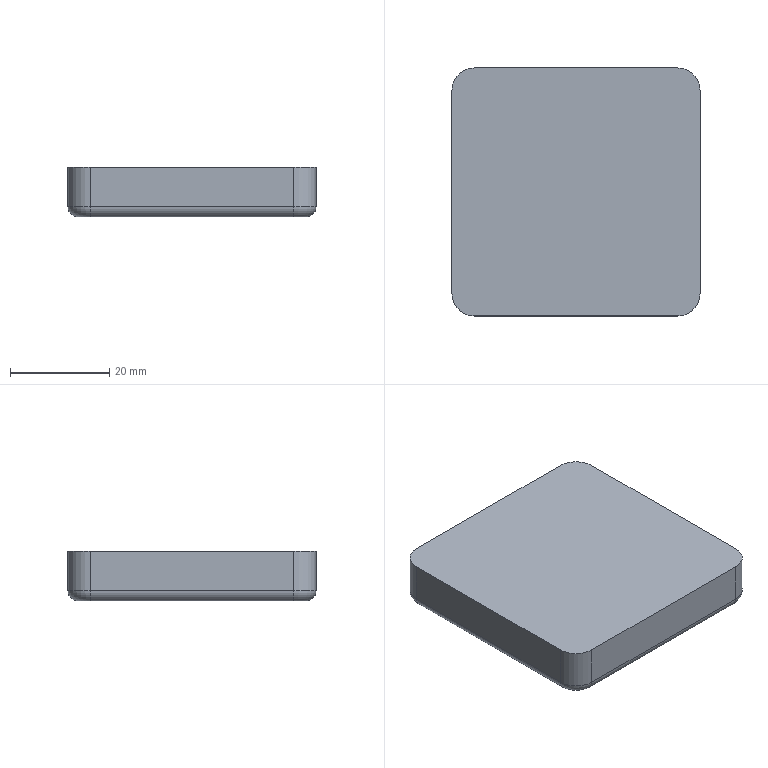Part | STEP file | 14831_CPY | 1 solid | 18 faces | box 50 x 50 x 10 mm | volume 24664 mm3 | cylinder 8 | plane 6 | torus 4 | commonest cylinder face diameters 4 x4 9 x4
STEP:
#1=CARTESIAN_POINT('',(0.,0.,0.));
#2=DIRECTION('',(0.,0.,1.));
#3=DIRECTION('',(1.,0.,0.));
#4=AXIS2_PLACEMENT_3D('',#1,#2,#3);
#5=CARTESIAN_POINT('',(-133.276,-146.636,0.));
#6=VERTEX_POINT('',#5);
#7=CARTESIAN_POINT('',(-133.276,-148.636,2.));
#8=VERTEX_POINT('',#7);
#9=CARTESIAN_POINT('',(-133.276,-146.636,2.));
#10=DIRECTION('',(-1.,0.,0.));
#11=DIRECTION('',(0.,0.,-1.));
#12=AXIS2_PLACEMENT_3D('',#9,#10,#11);
#13=CIRCLE('',#12,2.);
#14=CARTESIAN_POINT('',(-143.526,-146.636,2.));
#15=DIRECTION('',(-1.,0.,0.));
#16=DIRECTION('',(0.,-0.7071,-0.7071));
#17=AXIS2_PLACEMENT_3D('',#14,#15,#16);
#18=CYLINDRICAL_SURFACE('',#17,2.);
#19=CARTESIAN_POINT('',(5.498,-10.25));
#20=DIRECTION('',(1.,0.));
#21=VECTOR('',#20,1.);
#22=LINE('',#19,#21);
#23=(GEOMETRIC_REPRESENTATION_CONTEXT(2)PARAMETRIC_REPRESENTATION_CONTEXT()REPRESENTATION_CONTEXT('',''));
#24=DEFINITIONAL_REPRESENTATION('',(#22),#23);
#25=PCURVE('',#18,#24);
#26=CARTESIAN_POINT('',(-133.276,-144.136,2.));
#27=DIRECTION('',(0.,0.,-1.));
#28=DIRECTION('',(-1.,0.,0.));
#29=AXIS2_PLACEMENT_3D('',#26,#27,#28);
#30=TOROIDAL_SURFACE('',#29,2.5,2.);
#31=CARTESIAN_POINT('',(4.712,1.571));
#32=DIRECTION('',(0.,-1.));
#33=VECTOR('',#32,1.);
#34=LINE('',#31,#33);
#35=(GEOMETRIC_REPRESENTATION_CONTEXT(2)PARAMETRIC_REPRESENTATION_CONTEXT()REPRESENTATION_CONTEXT('',''));
#36=DEFINITIONAL_REPRESENTATION('',(#34),#35);
#37=PCURVE('',#30,#36);
#38=SURFACE_CURVE('',#13,(#25,#37),.PCURVE_S1.);
#39=EDGE_CURVE('',#6,#8,#38,.T.);
#40=ORIENTED_EDGE('',*,*,#39,.T.);
#41=CARTESIAN_POINT('',(-174.276,-148.636,2.));
#42=VERTEX_POINT('',#41);
#43=CARTESIAN_POINT('',(-133.276,-148.636,2.));
#44=DIRECTION('',(-1.,0.,0.));
#45=VECTOR('',#44,1.);
#46=LINE('',#43,#45);
#47=CARTESIAN_POINT('',(7.069,-10.25));
#48=DIRECTION('',(0.,1.));
#49=VECTOR('',#48,1.);
#50=LINE('',#47,#49);
#51=(GEOMETRIC_REPRESENTATION_CONTEXT(2)PARAMETRIC_REPRESENTATION_CONTEXT()REPRESENTATION_CONTEXT('',''));
#52=DEFINITIONAL_REPRESENTATION('',(#50),#51);
#53=PCURVE('',#18,#52);
#54=CARTESIAN_POINT('',(-133.276,-148.636,0.));
#55=DIRECTION('',(0.,-1.,0.));
#56=DIRECTION('',(0.,0.,-1.));
#57=AXIS2_PLACEMENT_3D('',#54,#55,#56);
#58=PLANE('',#57);
#59=CARTESIAN_POINT('',(-2.,0.));
#60=DIRECTION('',(0.,-1.));
#61=VECTOR('',#60,1.);
#62=LINE('',#59,#61);
#63=(GEOMETRIC_REPRESENTATION_CONTEXT(2)PARAMETRIC_REPRESENTATION_CONTEXT()REPRESENTATION_CONTEXT('',''));
#64=DEFINITIONAL_REPRESENTATION('',(#62),#63);
#65=PCURVE('',#58,#64);
#66=SURFACE_CURVE('',#46,(#53,#65),.PCURVE_S1.);
#67=EDGE_CURVE('',#8,#42,#66,.T.);
#68=ORIENTED_EDGE('',*,*,#67,.T.);
#69=CARTESIAN_POINT('',(-174.276,-146.636,0.));
#70=VERTEX_POINT('',#69);
#71=CARTESIAN_POINT('',(-174.276,-146.636,2.));
#72=DIRECTION('',(1.,0.,0.));
#73=DIRECTION('',(0.,-1.,0.));
#74=AXIS2_PLACEMENT_3D('',#71,#72,#73);
#75=CIRCLE('',#74,2.);
#76=CARTESIAN_POINT('',(7.069,30.75));
#77=DIRECTION('',(-1.,0.));
#78=VECTOR('',#77,1.);
#79=LINE('',#76,#78);
#80=(GEOMETRIC_REPRESENTATION_CONTEXT(2)PARAMETRIC_REPRESENTATION_CONTEXT()REPRESENTATION_CONTEXT('',''));
#81=DEFINITIONAL_REPRESENTATION('',(#79),#80);
#82=PCURVE('',#18,#81);
#83=CARTESIAN_POINT('',(-174.276,-144.136,2.));
#84=DIRECTION('',(0.,0.,-1.));
#85=DIRECTION('',(-1.,0.,0.));
#86=AXIS2_PLACEMENT_3D('',#83,#84,#85);
#87=TOROIDAL_SURFACE('',#86,2.5,2.);
#88=CARTESIAN_POINT('',(4.712,0.));
#89=DIRECTION('',(0.,1.));
#90=VECTOR('',#89,1.);
#91=LINE('',#88,#90);
#92=(GEOMETRIC_REPRESENTATION_CONTEXT(2)PARAMETRIC_REPRESENTATION_CONTEXT()REPRESENTATION_CONTEXT('',''));
#93=DEFINITIONAL_REPRESENTATION('',(#91),#92);
#94=PCURVE('',#87,#93);
#95=SURFACE_CURVE('',#75,(#82,#94),.PCURVE_S1.);
#96=EDGE_CURVE('',#42,#70,#95,.T.);
#97=ORIENTED_EDGE('',*,*,#96,.T.);
#98=CARTESIAN_POINT('',(-174.276,-146.636,0.));
#99=DIRECTION('',(1.,0.,0.));
#100=VECTOR('',#99,1.);
#101=LINE('',#98,#100);
#102=CARTESIAN_POINT('',(5.498,30.75));
#103=DIRECTION('',(0.,-1.));
#104=VECTOR('',#103,1.);
#105=LINE('',#102,#104);
#106=(GEOMETRIC_REPRESENTATION_CONTEXT(2)PARAMETRIC_REPRESENTATION_CONTEXT()REPRESENTATION_CONTEXT('',''));
#107=DEFINITIONAL_REPRESENTATION('',(#105),#106);
#108=PCURVE('',#18,#107);
#109=CARTESIAN_POINT('',(-153.776,-123.636,0.));
#110=DIRECTION('',(0.,0.,1.));
#111=DIRECTION('',(1.,0.,0.));
#112=AXIS2_PLACEMENT_3D('',#109,#110,#111);
#113=PLANE('',#112);
#114=CARTESIAN_POINT('',(-20.5,-23.));
#115=DIRECTION('',(1.,0.));
#116=VECTOR('',#115,1.);
#117=LINE('',#114,#116);
#118=(GEOMETRIC_REPRESENTATION_CONTEXT(2)PARAMETRIC_REPRESENTATION_CONTEXT()REPRESENTATION_CONTEXT('',''));
#119=DEFINITIONAL_REPRESENTATION('',(#117),#118);
#120=PCURVE('',#113,#119);
#121=SURFACE_CURVE('',#101,(#108,#120),.PCURVE_S1.);
#122=EDGE_CURVE('',#70,#6,#121,.T.);
#123=ORIENTED_EDGE('',*,*,#122,.T.);
#124=EDGE_LOOP('',(#40,#68,#97,#123));
#125=FACE_BOUND('',#124,.T.);
#126=ADVANCED_FACE('',(#125),#18,.T.);
#127=CARTESIAN_POINT('',(-130.776,-144.136,0.));
#128=VERTEX_POINT('',#127);
#129=CARTESIAN_POINT('',(-128.776,-144.136,2.));
#130=VERTEX_POINT('',#129);
#131=CARTESIAN_POINT('',(-130.776,-144.136,2.));
#132=DIRECTION('',(0.,-1.,0.));
#133=DIRECTION('',(0.,0.,-1.));
#134=AXIS2_PLACEMENT_3D('',#131,#132,#133);
#135=CIRCLE('',#134,2.);
#136=CARTESIAN_POINT('',(3.142,1.571));
#137=DIRECTION('',(0.,-1.));
#138=VECTOR('',#137,1.);
#139=LINE('',#136,#138);
#140=(GEOMETRIC_REPRESENTATION_CONTEXT(2)PARAMETRIC_REPRESENTATION_CONTEXT()REPRESENTATION_CONTEXT('',''));
#141=DEFINITIONAL_REPRESENTATION('',(#139),#140);
#142=PCURVE('',#30,#141);
#143=CARTESIAN_POINT('',(-130.776,-113.386,2.));
#144=DIRECTION('',(0.,-1.,0.));
#145=DIRECTION('',(0.7071,0.,-0.7071));
#146=AXIS2_PLACEMENT_3D('',#143,#144,#145);
#147=CYLINDRICAL_SURFACE('',#146,2.);
#148=CARTESIAN_POINT('',(5.498,30.75));
#149=DIRECTION('',(1.,0.));
#150=VECTOR('',#149,1.);
#151=LINE('',#148,#150);
#152=(GEOMETRIC_REPRESENTATION_CONTEXT(2)PARAMETRIC_REPRESENTATION_CONTEXT()REPRESENTATION_CONTEXT('',''));
#153=DEFINITIONAL_REPRESENTATION('',(#151),#152);
#154=PCURVE('',#147,#153);
#155=SURFACE_CURVE('',#135,(#142,#154),.PCURVE_S1.);
#156=EDGE_CURVE('',#128,#130,#155,.T.);
#157=ORIENTED_EDGE('',*,*,#156,.T.);
#158=CARTESIAN_POINT('',(-133.276,-144.136,2.));
#159=DIRECTION('',(0.,0.,-1.));
#160=DIRECTION('',(0.7071,-0.7071,0.));
#161=AXIS2_PLACEMENT_3D('',#158,#159,#160);
#162=CIRCLE('',#161,4.5);
#163=CARTESIAN_POINT('',(-2.356,0.));
#164=DIRECTION('',(1.,0.));
#165=VECTOR('',#164,1.);
#166=LINE('',#163,#165);
#167=(GEOMETRIC_REPRESENTATION_CONTEXT(2)PARAMETRIC_REPRESENTATION_CONTEXT()REPRESENTATION_CONTEXT('',''));
#168=DEFINITIONAL_REPRESENTATION('',(#166),#167);
#169=PCURVE('',#30,#168);
#170=CARTESIAN_POINT('',(-133.276,-144.136,0.));
#171=DIRECTION('',(0.,0.,1.));
#172=DIRECTION('',(0.,1.,0.));
#173=AXIS2_PLACEMENT_3D('',#170,#171,#172);
#174=CYLINDRICAL_SURFACE('',#173,4.5);
#175=CARTESIAN_POINT('',(10.21,2.));
#176=DIRECTION('',(-1.,0.));
#177=VECTOR('',#176,1.);
#178=LINE('',#175,#177);
#179=(GEOMETRIC_REPRESENTATION_CONTEXT(2)PARAMETRIC_REPRESENTATION_CONTEXT()REPRESENTATION_CONTEXT('',''));
#180=DEFINITIONAL_REPRESENTATION('',(#178),#179);
#181=PCURVE('',#174,#180);
#182=SURFACE_CURVE('',#162,(#169,#181),.PCURVE_S1.);
#183=EDGE_CURVE('',#130,#8,#182,.T.);
#184=ORIENTED_EDGE('',*,*,#183,.T.);
#185=ORIENTED_EDGE('',*,*,#39,.F.);
#186=CARTESIAN_POINT('',(-133.276,-144.136,0.));
#187=DIRECTION('',(0.,0.,1.));
#188=DIRECTION('',(0.7071,-0.7071,0.));
#189=AXIS2_PLACEMENT_3D('',#186,#187,#188);
#190=CIRCLE('',#189,2.5);
#191=CARTESIAN_POINT('',(10.21,1.571));
#192=DIRECTION('',(-1.,0.));
#193=VECTOR('',#192,1.);
#194=LINE('',#191,#193);
#195=(GEOMETRIC_REPRESENTATION_CONTEXT(2)PARAMETRIC_REPRESENTATION_CONTEXT()REPRESENTATION_CONTEXT('',''));
#196=DEFINITIONAL_REPRESENTATION('',(#194),#195);
#197=PCURVE('',#30,#196);
#198=CARTESIAN_POINT('',(20.5,-20.5));
#199=DIRECTION('',(0.7071,-0.7071));
#200=AXIS2_PLACEMENT_2D('',#198,#199);
#201=CIRCLE('',#200,2.5);
#202=(GEOMETRIC_REPRESENTATION_CONTEXT(2)PARAMETRIC_REPRESENTATION_CONTEXT()REPRESENTATION_CONTEXT('',''));
#203=DEFINITIONAL_REPRESENTATION('',(#201),#202);
#204=PCURVE('',#113,#203);
#205=SURFACE_CURVE('',#190,(#197,#204),.PCURVE_S1.);
#206=EDGE_CURVE('',#6,#128,#205,.T.);
#207=ORIENTED_EDGE('',*,*,#206,.T.);
#208=EDGE_LOOP('',(#157,#184,#185,#207));
#209=FACE_BOUND('',#208,.T.);
#210=ADVANCED_FACE('',(#209),#30,.T.);
#211=CARTESIAN_POINT('',(-178.776,-144.136,2.));
#212=VERTEX_POINT('',#211);
#213=CARTESIAN_POINT('',(-176.776,-144.136,0.));
#214=VERTEX_POINT('',#213);
#215=CARTESIAN_POINT('',(-176.776,-144.136,2.));
#216=DIRECTION('',(0.,-1.,0.));
#217=DIRECTION('',(-1.,0.,0.));
#218=AXIS2_PLACEMENT_3D('',#215,#216,#217);
#219=CIRCLE('',#218,2.);
#220=CARTESIAN_POINT('',(6.283,0.));
#221=DIRECTION('',(0.,1.));
#222=VECTOR('',#221,1.);
#223=LINE('',#220,#222);
#224=(GEOMETRIC_REPRESENTATION_CONTEXT(2)PARAMETRIC_REPRESENTATION_CONTEXT()REPRESENTATION_CONTEXT('',''));
#225=DEFINITIONAL_REPRESENTATION('',(#223),#224);
#226=PCURVE('',#87,#225);
#227=CARTESIAN_POINT('',(-176.776,-133.886,2.));
#228=DIRECTION('',(0.,1.,0.));
#229=DIRECTION('',(-0.7071,0.,-0.7071));
#230=AXIS2_PLACEMENT_3D('',#227,#228,#229);
#231=CYLINDRICAL_SURFACE('',#230,2.);
#232=CARTESIAN_POINT('',(7.069,-10.25));
#233=DIRECTION('',(-1.,0.));
#234=VECTOR('',#233,1.);
#235=LINE('',#232,#234);
#236=(GEOMETRIC_REPRESENTATION_CONTEXT(2)PARAMETRIC_REPRESENTATION_CONTEXT()REPRESENTATION_CONTEXT('',''));
#237=DEFINITIONAL_REPRESENTATION('',(#235),#236);
#238=PCURVE('',#231,#237);
#239=SURFACE_CURVE('',#219,(#226,#238),.PCURVE_S1.);
#240=EDGE_CURVE('',#212,#214,#239,.T.);
#241=ORIENTED_EDGE('',*,*,#240,.T.);
#242=CARTESIAN_POINT('',(-174.276,-144.136,0.));
#243=DIRECTION('',(0.,0.,1.));
#244=DIRECTION('',(-0.7071,-0.7071,0.));
#245=AXIS2_PLACEMENT_3D('',#242,#243,#244);
#246=CIRCLE('',#245,2.5);
#247=CARTESIAN_POINT('',(11.781,1.571));
#248=DIRECTION('',(-1.,0.));
#249=VECTOR('',#248,1.);
#250=LINE('',#247,#249);
#251=(GEOMETRIC_REPRESENTATION_CONTEXT(2)PARAMETRIC_REPRESENTATION_CONTEXT()REPRESENTATION_CONTEXT('',''));
#252=DEFINITIONAL_REPRESENTATION('',(#250),#251);
#253=PCURVE('',#87,#252);
#254=CARTESIAN_POINT('',(-20.5,-20.5));
#255=DIRECTION('',(-0.7071,-0.7071));
#256=AXIS2_PLACEMENT_2D('',#254,#255);
#257=CIRCLE('',#256,2.5);
#258=(GEOMETRIC_REPRESENTATION_CONTEXT(2)PARAMETRIC_REPRESENTATION_CONTEXT()REPRESENTATION_CONTEXT('',''));
#259=DEFINITIONAL_REPRESENTATION('',(#257),#258);
#260=PCURVE('',#113,#259);
#261=SURFACE_CURVE('',#246,(#253,#260),.PCURVE_S1.);
#262=EDGE_CURVE('',#214,#70,#261,.T.);
#263=ORIENTED_EDGE('',*,*,#262,.T.);
#264=ORIENTED_EDGE('',*,*,#96,.F.);
#265=CARTESIAN_POINT('',(-174.276,-144.136,2.));
#266=DIRECTION('',(0.,0.,-1.));
#267=DIRECTION('',(-0.7071,-0.7071,0.));
#268=AXIS2_PLACEMENT_3D('',#265,#266,#267);
#269=CIRCLE('',#268,4.5);
#270=CARTESIAN_POINT('',(-0.7854,0.));
#271=DIRECTION('',(1.,0.));
#272=VECTOR('',#271,1.);
#273=LINE('',#270,#272);
#274=(GEOMETRIC_REPRESENTATION_CONTEXT(2)PARAMETRIC_REPRESENTATION_CONTEXT()REPRESENTATION_CONTEXT('',''));
#275=DEFINITIONAL_REPRESENTATION('',(#273),#274);
#276=PCURVE('',#87,#275);
#277=CARTESIAN_POINT('',(-174.276,-144.136,0.));
#278=DIRECTION('',(0.,0.,1.));
#279=DIRECTION('',(1.,0.,0.));
#280=AXIS2_PLACEMENT_3D('',#277,#278,#279);
#281=CYLINDRICAL_SURFACE('',#280,4.5);
#282=CARTESIAN_POINT('',(10.21,2.));
#283=DIRECTION('',(-1.,0.));
#284=VECTOR('',#283,1.);
#285=LINE('',#282,#284);
#286=(GEOMETRIC_REPRESENTATION_CONTEXT(2)PARAMETRIC_REPRESENTATION_CONTEXT()REPRESENTATION_CONTEXT('',''));
#287=DEFINITIONAL_REPRESENTATION('',(#285),#286);
#288=PCURVE('',#281,#287);
#289=SURFACE_CURVE('',#269,(#276,#288),.PCURVE_S1.);
#290=EDGE_CURVE('',#42,#212,#289,.T.);
#291=ORIENTED_EDGE('',*,*,#290,.T.);
#292=EDGE_LOOP('',(#241,#263,#264,#291));
#293=FACE_BOUND('',#292,.T.);
#294=ADVANCED_FACE('',(#293),#87,.T.);
#295=CARTESIAN_POINT('',(-130.776,-103.136,0.));
#296=VERTEX_POINT('',#295);
#297=CARTESIAN_POINT('',(-128.776,-103.136,2.));
#298=VERTEX_POINT('',#297);
#299=CARTESIAN_POINT('',(-130.776,-103.136,2.));
#300=DIRECTION('',(0.,-1.,0.));
#301=DIRECTION('',(0.,0.,-1.));
#302=AXIS2_PLACEMENT_3D('',#299,#300,#301);
#303=CIRCLE('',#302,2.);
#304=CARTESIAN_POINT('',(5.498,-10.25));
#305=DIRECTION('',(1.,0.));
#306=VECTOR('',#305,1.);
#307=LINE('',#304,#306);
#308=(GEOMETRIC_REPRESENTATION_CONTEXT(2)PARAMETRIC_REPRESENTATION_CONTEXT()REPRESENTATION_CONTEXT('',''));
#309=DEFINITIONAL_REPRESENTATION('',(#307),#308);
#310=PCURVE('',#147,#309);
#311=CARTESIAN_POINT('',(-133.276,-103.136,2.));
#312=DIRECTION('',(0.,0.,-1.));
#313=DIRECTION('',(-1.,0.,0.));
#314=AXIS2_PLACEMENT_3D('',#311,#312,#313);
#315=TOROIDAL_SURFACE('',#314,2.5,2.);
#316=CARTESIAN_POINT('',(3.142,1.571));
#317=DIRECTION('',(0.,-1.));
#318=VECTOR('',#317,1.);
#319=LINE('',#316,#318);
#320=(GEOMETRIC_REPRESENTATION_CONTEXT(2)PARAMETRIC_REPRESENTATION_CONTEXT()REPRESENTATION_CONTEXT('',''));
#321=DEFINITIONAL_REPRESENTATION('',(#319),#320);
#322=PCURVE('',#315,#321);
#323=SURFACE_CURVE('',#303,(#310,#322),.PCURVE_S1.);
#324=EDGE_CURVE('',#296,#298,#323,.T.);
#325=ORIENTED_EDGE('',*,*,#324,.T.);
#326=CARTESIAN_POINT('',(-128.776,-103.136,2.));
#327=DIRECTION('',(0.,-1.,0.));
#328=VECTOR('',#327,1.);
#329=LINE('',#326,#328);
#330=CARTESIAN_POINT('',(7.069,-10.25));
#331=DIRECTION('',(0.,1.));
#332=VECTOR('',#331,1.);
#333=LINE('',#330,#332);
#334=(GEOMETRIC_REPRESENTATION_CONTEXT(2)PARAMETRIC_REPRESENTATION_CONTEXT()REPRESENTATION_CONTEXT('',''));
#335=DEFINITIONAL_REPRESENTATION('',(#333),#334);
#336=PCURVE('',#147,#335);
#337=CARTESIAN_POINT('',(-128.776,-103.136,0.));
#338=DIRECTION('',(1.,0.,0.));
#339=DIRECTION('',(0.,0.,-1.));
#340=AXIS2_PLACEMENT_3D('',#337,#338,#339);
#341=PLANE('',#340);
#342=CARTESIAN_POINT('',(-2.,0.));
#343=DIRECTION('',(0.,-1.));
#344=VECTOR('',#343,1.);
#345=LINE('',#342,#344);
#346=(GEOMETRIC_REPRESENTATION_CONTEXT(2)PARAMETRIC_REPRESENTATION_CONTEXT()REPRESENTATION_CONTEXT('',''));
#347=DEFINITIONAL_REPRESENTATION('',(#345),#346);
#348=PCURVE('',#341,#347);
#349=SURFACE_CURVE('',#329,(#336,#348),.PCURVE_S1.);
#350=EDGE_CURVE('',#298,#130,#349,.T.);
#351=ORIENTED_EDGE('',*,*,#350,.T.);
#352=ORIENTED_EDGE('',*,*,#156,.F.);
#353=CARTESIAN_POINT('',(-130.776,-144.136,0.));
#354=DIRECTION('',(0.,1.,0.));
#355=VECTOR('',#354,1.);
#356=LINE('',#353,#355);
#357=CARTESIAN_POINT('',(5.498,30.75));
#358=DIRECTION('',(0.,-1.));
#359=VECTOR('',#358,1.);
#360=LINE('',#357,#359);
#361=(GEOMETRIC_REPRESENTATION_CONTEXT(2)PARAMETRIC_REPRESENTATION_CONTEXT()REPRESENTATION_CONTEXT('',''));
#362=DEFINITIONAL_REPRESENTATION('',(#360),#361);
#363=PCURVE('',#147,#362);
#364=CARTESIAN_POINT('',(23.,-20.5));
#365=DIRECTION('',(0.,1.));
#366=VECTOR('',#365,1.);
#367=LINE('',#364,#366);
#368=(GEOMETRIC_REPRESENTATION_CONTEXT(2)PARAMETRIC_REPRESENTATION_CONTEXT()REPRESENTATION_CONTEXT('',''));
#369=DEFINITIONAL_REPRESENTATION('',(#367),#368);
#370=PCURVE('',#113,#369);
#371=SURFACE_CURVE('',#356,(#363,#370),.PCURVE_S1.);
#372=EDGE_CURVE('',#128,#296,#371,.T.);
#373=ORIENTED_EDGE('',*,*,#372,.T.);
#374=EDGE_LOOP('',(#325,#351,#352,#373));
#375=FACE_BOUND('',#374,.T.);
#376=ADVANCED_FACE('',(#375),#147,.T.);
#377=CARTESIAN_POINT('',(-178.776,-103.136,2.));
#378=VERTEX_POINT('',#377);
#379=CARTESIAN_POINT('',(-176.776,-103.136,0.));
#380=VERTEX_POINT('',#379);
#381=CARTESIAN_POINT('',(-176.776,-103.136,2.));
#382=DIRECTION('',(0.,-1.,0.));
#383=DIRECTION('',(-1.,0.,0.));
#384=AXIS2_PLACEMENT_3D('',#381,#382,#383);
#385=CIRCLE('',#384,2.);
#386=CARTESIAN_POINT('',(7.069,30.75));
#387=DIRECTION('',(-1.,0.));
#388=VECTOR('',#387,1.);
#389=LINE('',#386,#388);
#390=(GEOMETRIC_REPRESENTATION_CONTEXT(2)PARAMETRIC_REPRESENTATION_CONTEXT()REPRESENTATION_CONTEXT('',''));
#391=DEFINITIONAL_REPRESENTATION('',(#389),#390);
#392=PCURVE('',#231,#391);
#393=CARTESIAN_POINT('',(-174.276,-103.136,2.));
#394=DIRECTION('',(0.,0.,-1.));
#395=DIRECTION('',(-1.,0.,0.));
#396=AXIS2_PLACEMENT_3D('',#393,#394,#395);
#397=TOROIDAL_SURFACE('',#396,2.5,2.);
#398=CARTESIAN_POINT('',(0.,0.));
#399=DIRECTION('',(0.,1.));
#400=VECTOR('',#399,1.);
#401=LINE('',#398,#400);
#402=(GEOMETRIC_REPRESENTATION_CONTEXT(2)PARAMETRIC_REPRESENTATION_CONTEXT()REPRESENTATION_CONTEXT('',''));
#403=DEFINITIONAL_REPRESENTATION('',(#401),#402);
#404=PCURVE('',#397,#403);
#405=SURFACE_CURVE('',#385,(#392,#404),.PCURVE_S1.);
#406=EDGE_CURVE('',#378,#380,#405,.T.);
#407=ORIENTED_EDGE('',*,*,#406,.T.);
#408=CARTESIAN_POINT('',(-176.776,-103.136,0.));
#409=DIRECTION('',(0.,-1.,0.));
#410=VECTOR('',#409,1.);
#411=LINE('',#408,#410);
#412=CARTESIAN_POINT('',(5.498,30.75));
#413=DIRECTION('',(0.,-1.));
#414=VECTOR('',#413,1.);
#415=LINE('',#412,#414);
#416=(GEOMETRIC_REPRESENTATION_CONTEXT(2)PARAMETRIC_REPRESENTATION_CONTEXT()REPRESENTATION_CONTEXT('',''));
#417=DEFINITIONAL_REPRESENTATION('',(#415),#416);
#418=PCURVE('',#231,#417);
#419=CARTESIAN_POINT('',(-23.,20.5));
#420=DIRECTION('',(0.,-1.));
#421=VECTOR('',#420,1.);
#422=LINE('',#419,#421);
#423=(GEOMETRIC_REPRESENTATION_CONTEXT(2)PARAMETRIC_REPRESENTATION_CONTEXT()REPRESENTATION_CONTEXT('',''));
#424=DEFINITIONAL_REPRESENTATION('',(#422),#423);
#425=PCURVE('',#113,#424);
#426=SURFACE_CURVE('',#411,(#418,#425),.PCURVE_S1.);
#427=EDGE_CURVE('',#380,#214,#426,.T.);
#428=ORIENTED_EDGE('',*,*,#427,.T.);
#429=ORIENTED_EDGE('',*,*,#240,.F.);
#430=CARTESIAN_POINT('',(-178.776,-144.136,2.));
#431=DIRECTION('',(0.,1.,0.));
#432=VECTOR('',#431,1.);
#433=LINE('',#430,#432);
#434=CARTESIAN_POINT('',(7.069,-10.25));
#435=DIRECTION('',(0.,1.));
#436=VECTOR('',#435,1.);
#437=LINE('',#434,#436);
#438=(GEOMETRIC_REPRESENTATION_CONTEXT(2)PARAMETRIC_REPRESENTATION_CONTEXT()REPRESENTATION_CONTEXT('',''));
#439=DEFINITIONAL_REPRESENTATION('',(#437),#438);
#440=PCURVE('',#231,#439);
#441=CARTESIAN_POINT('',(-178.776,-144.136,0.));
#442=DIRECTION('',(-1.,0.,0.));
#443=DIRECTION('',(0.,0.,1.));
#444=AXIS2_PLACEMENT_3D('',#441,#442,#443);
#445=PLANE('',#444);
#446=CARTESIAN_POINT('',(2.,0.));
#447=DIRECTION('',(0.,1.));
#448=VECTOR('',#447,1.);
#449=LINE('',#446,#448);
#450=(GEOMETRIC_REPRESENTATION_CONTEXT(2)PARAMETRIC_REPRESENTATION_CONTEXT()REPRESENTATION_CONTEXT('',''));
#451=DEFINITIONAL_REPRESENTATION('',(#449),#450);
#452=PCURVE('',#445,#451);
#453=SURFACE_CURVE('',#433,(#440,#452),.PCURVE_S1.);
#454=EDGE_CURVE('',#212,#378,#453,.T.);
#455=ORIENTED_EDGE('',*,*,#454,.T.);
#456=EDGE_LOOP('',(#407,#428,#429,#455));
#457=FACE_BOUND('',#456,.T.);
#458=ADVANCED_FACE('',(#457),#231,.T.);
#459=CARTESIAN_POINT('',(-133.276,-100.636,0.));
#460=VERTEX_POINT('',#459);
#461=CARTESIAN_POINT('',(-133.276,-98.636,2.));
#462=VERTEX_POINT('',#461);
#463=CARTESIAN_POINT('',(-133.276,-100.636,2.));
#464=DIRECTION('',(1.,0.,0.));
#465=DIRECTION('',(0.,0.,-1.));
#466=AXIS2_PLACEMENT_3D('',#463,#464,#465);
#467=CIRCLE('',#466,2.);
#468=CARTESIAN_POINT('',(1.571,1.571));
#469=DIRECTION('',(0.,-1.));
#470=VECTOR('',#469,1.);
#471=LINE('',#468,#470);
#472=(GEOMETRIC_REPRESENTATION_CONTEXT(2)PARAMETRIC_REPRESENTATION_CONTEXT()REPRESENTATION_CONTEXT('',''));
#473=DEFINITIONAL_REPRESENTATION('',(#471),#472);
#474=PCURVE('',#315,#473);
#475=CARTESIAN_POINT('',(-164.026,-100.636,2.));
#476=DIRECTION('',(1.,0.,0.));
#477=DIRECTION('',(0.,0.7071,-0.7071));
#478=AXIS2_PLACEMENT_3D('',#475,#476,#477);
#479=CYLINDRICAL_SURFACE('',#478,2.);
#480=CARTESIAN_POINT('',(5.498,30.75));
#481=DIRECTION('',(1.,0.));
#482=VECTOR('',#481,1.);
#483=LINE('',#480,#482);
#484=(GEOMETRIC_REPRESENTATION_CONTEXT(2)PARAMETRIC_REPRESENTATION_CONTEXT()REPRESENTATION_CONTEXT('',''));
#485=DEFINITIONAL_REPRESENTATION('',(#483),#484);
#486=PCURVE('',#479,#485);
#487=SURFACE_CURVE('',#467,(#474,#486),.PCURVE_S1.);
#488=EDGE_CURVE('',#460,#462,#487,.T.);
#489=ORIENTED_EDGE('',*,*,#488,.T.);
#490=CARTESIAN_POINT('',(-133.276,-103.136,2.));
#491=DIRECTION('',(0.,0.,-1.));
#492=DIRECTION('',(0.7071,0.7071,0.));
#493=AXIS2_PLACEMENT_3D('',#490,#491,#492);
#494=CIRCLE('',#493,4.5);
#495=CARTESIAN_POINT('',(-3.927,0.));
#496=DIRECTION('',(1.,0.));
#497=VECTOR('',#496,1.);
#498=LINE('',#495,#497);
#499=(GEOMETRIC_REPRESENTATION_CONTEXT(2)PARAMETRIC_REPRESENTATION_CONTEXT()REPRESENTATION_CONTEXT('',''));
#500=DEFINITIONAL_REPRESENTATION('',(#498),#499);
#501=PCURVE('',#315,#500);
#502=CARTESIAN_POINT('',(-133.276,-103.136,0.));
#503=DIRECTION('',(0.,0.,1.));
#504=DIRECTION('',(-1.,0.,0.));
#505=AXIS2_PLACEMENT_3D('',#502,#503,#504);
#506=CYLINDRICAL_SURFACE('',#505,4.5);
#507=CARTESIAN_POINT('',(10.21,2.));
#508=DIRECTION('',(-1.,0.));
#509=VECTOR('',#508,1.);
#510=LINE('',#507,#509);
#511=(GEOMETRIC_REPRESENTATION_CONTEXT(2)PARAMETRIC_REPRESENTATION_CONTEXT()REPRESENTATION_CONTEXT('',''));
#512=DEFINITIONAL_REPRESENTATION('',(#510),#511);
#513=PCURVE('',#506,#512);
#514=SURFACE_CURVE('',#494,(#501,#513),.PCURVE_S1.);
#515=EDGE_CURVE('',#462,#298,#514,.T.);
#516=ORIENTED_EDGE('',*,*,#515,.T.);
#517=ORIENTED_EDGE('',*,*,#324,.F.);
#518=CARTESIAN_POINT('',(-133.276,-103.136,0.));
#519=DIRECTION('',(0.,0.,1.));
#520=DIRECTION('',(0.7071,0.7071,0.));
#521=AXIS2_PLACEMENT_3D('',#518,#519,#520);
#522=CIRCLE('',#521,2.5);
#523=CARTESIAN_POINT('',(8.639,1.571));
#524=DIRECTION('',(-1.,0.));
#525=VECTOR('',#524,1.);
#526=LINE('',#523,#525);
#527=(GEOMETRIC_REPRESENTATION_CONTEXT(2)PARAMETRIC_REPRESENTATION_CONTEXT()REPRESENTATION_CONTEXT('',''));
#528=DEFINITIONAL_REPRESENTATION('',(#526),#527);
#529=PCURVE('',#315,#528);
#530=CARTESIAN_POINT('',(20.5,20.5));
#531=DIRECTION('',(0.7071,0.7071));
#532=AXIS2_PLACEMENT_2D('',#530,#531);
#533=CIRCLE('',#532,2.5);
#534=(GEOMETRIC_REPRESENTATION_CONTEXT(2)PARAMETRIC_REPRESENTATION_CONTEXT()REPRESENTATION_CONTEXT('',''));
#535=DEFINITIONAL_REPRESENTATION('',(#533),#534);
#536=PCURVE('',#113,#535);
#537=SURFACE_CURVE('',#522,(#529,#536),.PCURVE_S1.);
#538=EDGE_CURVE('',#296,#460,#537,.T.);
#539=ORIENTED_EDGE('',*,*,#538,.T.);
#540=EDGE_LOOP('',(#489,#516,#517,#539));
#541=FACE_BOUND('',#540,.T.);
#542=ADVANCED_FACE('',(#541),#315,.T.);
#543=CARTESIAN_POINT('',(-174.276,-98.636,2.));
#544=VERTEX_POINT('',#543);
#545=CARTESIAN_POINT('',(-174.276,-100.636,0.));
#546=VERTEX_POINT('',#545);
#547=CARTESIAN_POINT('',(-174.276,-100.636,2.));
#548=DIRECTION('',(-1.,0.,0.));
#549=DIRECTION('',(0.,1.,0.));
#550=AXIS2_PLACEMENT_3D('',#547,#548,#549);
#551=CIRCLE('',#550,2.);
#552=CARTESIAN_POINT('',(1.571,0.));
#553=DIRECTION('',(0.,1.));
#554=VECTOR('',#553,1.);
#555=LINE('',#552,#554);
#556=(GEOMETRIC_REPRESENTATION_CONTEXT(2)PARAMETRIC_REPRESENTATION_CONTEXT()REPRESENTATION_CONTEXT('',''));
#557=DEFINITIONAL_REPRESENTATION('',(#555),#556);
#558=PCURVE('',#397,#557);
#559=CARTESIAN_POINT('',(7.069,-10.25));
#560=DIRECTION('',(-1.,0.));
#561=VECTOR('',#560,1.);
#562=LINE('',#559,#561);
#563=(GEOMETRIC_REPRESENTATION_CONTEXT(2)PARAMETRIC_REPRESENTATION_CONTEXT()REPRESENTATION_CONTEXT('',''));
#564=DEFINITIONAL_REPRESENTATION('',(#562),#563);
#565=PCURVE('',#479,#564);
#566=SURFACE_CURVE('',#551,(#558,#565),.PCURVE_S1.);
#567=EDGE_CURVE('',#544,#546,#566,.T.);
#568=ORIENTED_EDGE('',*,*,#567,.T.);
#569=CARTESIAN_POINT('',(-174.276,-103.136,0.));
#570=DIRECTION('',(0.,0.,1.));
#571=DIRECTION('',(-0.7071,0.7071,0.));
#572=AXIS2_PLACEMENT_3D('',#569,#570,#571);
#573=CIRCLE('',#572,2.5);
#574=CARTESIAN_POINT('',(7.069,1.571));
#575=DIRECTION('',(-1.,0.));
#576=VECTOR('',#575,1.);
#577=LINE('',#574,#576);
#578=(GEOMETRIC_REPRESENTATION_CONTEXT(2)PARAMETRIC_REPRESENTATION_CONTEXT()REPRESENTATION_CONTEXT('',''));
#579=DEFINITIONAL_REPRESENTATION('',(#577),#578);
#580=PCURVE('',#397,#579);
#581=CARTESIAN_POINT('',(-20.5,20.5));
#582=DIRECTION('',(-0.7071,0.7071));
#583=AXIS2_PLACEMENT_2D('',#581,#582);
#584=CIRCLE('',#583,2.5);
#585=(GEOMETRIC_REPRESENTATION_CONTEXT(2)PARAMETRIC_REPRESENTATION_CONTEXT()REPRESENTATION_CONTEXT('',''));
#586=DEFINITIONAL_REPRESENTATION('',(#584),#585);
#587=PCURVE('',#113,#586);
#588=SURFACE_CURVE('',#573,(#580,#587),.PCURVE_S1.);
#589=EDGE_CURVE('',#546,#380,#588,.T.);
#590=ORIENTED_EDGE('',*,*,#589,.T.);
#591=ORIENTED_EDGE('',*,*,#406,.F.);
#592=CARTESIAN_POINT('',(-174.276,-103.136,2.));
#593=DIRECTION('',(0.,0.,-1.));
#594=DIRECTION('',(-0.7071,0.7071,0.));
#595=AXIS2_PLACEMENT_3D('',#592,#593,#594);
#596=CIRCLE('',#595,4.5);
#597=CARTESIAN_POINT('',(-5.498,0.));
#598=DIRECTION('',(1.,0.));
#599=VECTOR('',#598,1.);
#600=LINE('',#597,#599);
#601=(GEOMETRIC_REPRESENTATION_CONTEXT(2)PARAMETRIC_REPRESENTATION_CONTEXT()REPRESENTATION_CONTEXT('',''));
#602=DEFINITIONAL_REPRESENTATION('',(#600),#601);
#603=PCURVE('',#397,#602);
#604=CARTESIAN_POINT('',(-174.276,-103.136,0.));
#605=DIRECTION('',(0.,0.,1.));
#606=DIRECTION('',(0.,-1.,0.));
#607=AXIS2_PLACEMENT_3D('',#604,#605,#606);
#608=CYLINDRICAL_SURFACE('',#607,4.5);
#609=CARTESIAN_POINT('',(10.21,2.));
#610=DIRECTION('',(-1.,0.));
#611=VECTOR('',#610,1.);
#612=LINE('',#609,#611);
#613=(GEOMETRIC_REPRESENTATION_CONTEXT(2)PARAMETRIC_REPRESENTATION_CONTEXT()REPRESENTATION_CONTEXT('',''));
#614=DEFINITIONAL_REPRESENTATION('',(#612),#613);
#615=PCURVE('',#608,#614);
#616=SURFACE_CURVE('',#596,(#603,#615),.PCURVE_S1.);
#617=EDGE_CURVE('',#378,#544,#616,.T.);
#618=ORIENTED_EDGE('',*,*,#617,.T.);
#619=EDGE_LOOP('',(#568,#590,#591,#618));
#620=FACE_BOUND('',#619,.T.);
#621=ADVANCED_FACE('',(#620),#397,.T.);
#622=ORIENTED_EDGE('',*,*,#488,.F.);
#623=CARTESIAN_POINT('',(-133.276,-100.636,0.));
#624=DIRECTION('',(-1.,0.,0.));
#625=VECTOR('',#624,1.);
#626=LINE('',#623,#625);
#627=CARTESIAN_POINT('',(5.498,30.75));
#628=DIRECTION('',(0.,-1.));
#629=VECTOR('',#628,1.);
#630=LINE('',#627,#629);
#631=(GEOMETRIC_REPRESENTATION_CONTEXT(2)PARAMETRIC_REPRESENTATION_CONTEXT()REPRESENTATION_CONTEXT('',''));
#632=DEFINITIONAL_REPRESENTATION('',(#630),#631);
#633=PCURVE('',#479,#632);
#634=CARTESIAN_POINT('',(20.5,23.));
#635=DIRECTION('',(-1.,0.));
#636=VECTOR('',#635,1.);
#637=LINE('',#634,#636);
#638=(GEOMETRIC_REPRESENTATION_CONTEXT(2)PARAMETRIC_REPRESENTATION_CONTEXT()REPRESENTATION_CONTEXT('',''));
#639=DEFINITIONAL_REPRESENTATION('',(#637),#638);
#640=PCURVE('',#113,#639);
#641=SURFACE_CURVE('',#626,(#633,#640),.PCURVE_S1.);
#642=EDGE_CURVE('',#460,#546,#641,.T.);
#643=ORIENTED_EDGE('',*,*,#642,.T.);
#644=ORIENTED_EDGE('',*,*,#567,.F.);
#645=CARTESIAN_POINT('',(-174.276,-98.636,2.));
#646=DIRECTION('',(1.,0.,0.));
#647=VECTOR('',#646,1.);
#648=LINE('',#645,#647);
#649=CARTESIAN_POINT('',(7.069,-10.25));
#650=DIRECTION('',(0.,1.));
#651=VECTOR('',#650,1.);
#652=LINE('',#649,#651);
#653=(GEOMETRIC_REPRESENTATION_CONTEXT(2)PARAMETRIC_REPRESENTATION_CONTEXT()REPRESENTATION_CONTEXT('',''));
#654=DEFINITIONAL_REPRESENTATION('',(#652),#653);
#655=PCURVE('',#479,#654);
#656=CARTESIAN_POINT('',(-174.276,-98.636,0.));
#657=DIRECTION('',(0.,1.,0.));
#658=DIRECTION('',(0.,0.,1.));
#659=AXIS2_PLACEMENT_3D('',#656,#657,#658);
#660=PLANE('',#659);
#661=CARTESIAN_POINT('',(2.,0.));
#662=DIRECTION('',(0.,1.));
#663=VECTOR('',#662,1.);
#664=LINE('',#661,#663);
#665=(GEOMETRIC_REPRESENTATION_CONTEXT(2)PARAMETRIC_REPRESENTATION_CONTEXT()REPRESENTATION_CONTEXT('',''));
#666=DEFINITIONAL_REPRESENTATION('',(#664),#665);
#667=PCURVE('',#660,#666);
#668=SURFACE_CURVE('',#648,(#655,#667),.PCURVE_S1.);
#669=EDGE_CURVE('',#544,#462,#668,.T.);
#670=ORIENTED_EDGE('',*,*,#669,.T.);
#671=EDGE_LOOP('',(#622,#643,#644,#670));
#672=FACE_BOUND('',#671,.T.);
#673=ADVANCED_FACE('',(#672),#479,.T.);
#674=ORIENTED_EDGE('',*,*,#617,.F.);
#675=CARTESIAN_POINT('',(-178.776,-103.136,10.));
#676=VERTEX_POINT('',#675);
#677=CARTESIAN_POINT('',(-178.776,-103.136,2.));
#678=DIRECTION('',(0.,0.,1.));
#679=VECTOR('',#678,1.);
#680=LINE('',#677,#679);
#681=CARTESIAN_POINT('',(4.712,2.));
#682=DIRECTION('',(0.,1.));
#683=VECTOR('',#682,1.);
#684=LINE('',#681,#683);
#685=(GEOMETRIC_REPRESENTATION_CONTEXT(2)PARAMETRIC_REPRESENTATION_CONTEXT()REPRESENTATION_CONTEXT('',''));
#686=DEFINITIONAL_REPRESENTATION('',(#684),#685);
#687=PCURVE('',#608,#686);
#688=CARTESIAN_POINT('',(2.,41.));
#689=DIRECTION('',(1.,0.));
#690=VECTOR('',#689,1.);
#691=LINE('',#688,#690);
#692=(GEOMETRIC_REPRESENTATION_CONTEXT(2)PARAMETRIC_REPRESENTATION_CONTEXT()REPRESENTATION_CONTEXT('',''));
#693=DEFINITIONAL_REPRESENTATION('',(#691),#692);
#694=PCURVE('',#445,#693);
#695=SURFACE_CURVE('',#680,(#687,#694),.PCURVE_S1.);
#696=EDGE_CURVE('',#378,#676,#695,.T.);
#697=ORIENTED_EDGE('',*,*,#696,.T.);
#698=CARTESIAN_POINT('',(-174.276,-98.636,10.));
#699=VERTEX_POINT('',#698);
#700=CARTESIAN_POINT('',(-174.276,-103.136,10.));
#701=DIRECTION('',(0.,0.,-1.));
#702=DIRECTION('',(0.,-1.,0.));
#703=AXIS2_PLACEMENT_3D('',#700,#701,#702);
#704=CIRCLE('',#703,4.5);
#705=CARTESIAN_POINT('',(6.283,10.));
#706=DIRECTION('',(-1.,0.));
#707=VECTOR('',#706,1.);
#708=LINE('',#705,#707);
#709=(GEOMETRIC_REPRESENTATION_CONTEXT(2)PARAMETRIC_REPRESENTATION_CONTEXT()REPRESENTATION_CONTEXT('',''));
#710=DEFINITIONAL_REPRESENTATION('',(#708),#709);
#711=PCURVE('',#608,#710);
#712=CARTESIAN_POINT('',(-153.776,-123.636,10.));
#713=DIRECTION('',(0.,0.,1.));
#714=DIRECTION('',(1.,0.,0.));
#715=AXIS2_PLACEMENT_3D('',#712,#713,#714);
#716=PLANE('',#715);
#717=CARTESIAN_POINT('',(-20.5,16.));
#718=CARTESIAN_POINT('',(-28.294,16.));
#719=CARTESIAN_POINT('',(-24.397,22.75));
#720=CARTESIAN_POINT('',(-20.5,29.5));
#721=CARTESIAN_POINT('',(-16.603,22.75));
#722=CARTESIAN_POINT('',(-12.706,16.));
#723=CARTESIAN_POINT('',(-20.5,16.));
#724=(BOUNDED_CURVE()B_SPLINE_CURVE(2,(#717,#718,#719,#720,#721,#722,#723),.UNSPECIFIED.,.T.,.F.)B_SPLINE_CURVE_WITH_KNOTS((1,2,2,2,2,1),(-2.094,0.,2.094,4.189,6.283,8.378),.UNSPECIFIED.)CURVE()GEOMETRIC_REPRESENTATION_ITEM()RATIONAL_B_SPLINE_CURVE((1.,0.5,1.,0.5,1.,0.5,1.))REPRESENTATION_ITEM(''));
#725=(GEOMETRIC_REPRESENTATION_CONTEXT(2)PARAMETRIC_REPRESENTATION_CONTEXT()REPRESENTATION_CONTEXT('',''));
#726=DEFINITIONAL_REPRESENTATION('',(#724),#725);
#727=PCURVE('',#716,#726);
#728=SURFACE_CURVE('',#704,(#711,#727),.PCURVE_S1.);
#729=EDGE_CURVE('',#676,#699,#728,.T.);
#730=ORIENTED_EDGE('',*,*,#729,.T.);
#731=CARTESIAN_POINT('',(-174.276,-98.636,2.));
#732=DIRECTION('',(0.,0.,1.));
#733=VECTOR('',#732,1.);
#734=LINE('',#731,#733);
#735=CARTESIAN_POINT('',(3.142,2.));
#736=DIRECTION('',(0.,1.));
#737=VECTOR('',#736,1.);
#738=LINE('',#735,#737);
#739=(GEOMETRIC_REPRESENTATION_CONTEXT(2)PARAMETRIC_REPRESENTATION_CONTEXT()REPRESENTATION_CONTEXT('',''));
#740=DEFINITIONAL_REPRESENTATION('',(#738),#739);
#741=PCURVE('',#608,#740);
#742=CARTESIAN_POINT('',(2.,0.));
#743=DIRECTION('',(1.,0.));
#744=VECTOR('',#743,1.);
#745=LINE('',#742,#744);
#746=(GEOMETRIC_REPRESENTATION_CONTEXT(2)PARAMETRIC_REPRESENTATION_CONTEXT()REPRESENTATION_CONTEXT('',''));
#747=DEFINITIONAL_REPRESENTATION('',(#745),#746);
#748=PCURVE('',#660,#747);
#749=SURFACE_CURVE('',#734,(#741,#748),.PCURVE_S1.);
#750=EDGE_CURVE('',#544,#699,#749,.T.);
#751=ORIENTED_EDGE('',*,*,#750,.F.);
#752=EDGE_LOOP('',(#674,#697,#730,#751));
#753=FACE_BOUND('',#752,.T.);
#754=ADVANCED_FACE('',(#753),#608,.T.);
#755=ORIENTED_EDGE('',*,*,#454,.F.);
#756=CARTESIAN_POINT('',(-178.776,-144.136,10.));
#757=VERTEX_POINT('',#756);
#758=CARTESIAN_POINT('',(-178.776,-144.136,2.));
#759=DIRECTION('',(0.,0.,1.));
#760=VECTOR('',#759,1.);
#761=LINE('',#758,#760);
#762=CARTESIAN_POINT('',(2.,0.));
#763=DIRECTION('',(1.,0.));
#764=VECTOR('',#763,1.);
#765=LINE('',#762,#764);
#766=(GEOMETRIC_REPRESENTATION_CONTEXT(2)PARAMETRIC_REPRESENTATION_CONTEXT()REPRESENTATION_CONTEXT('',''));
#767=DEFINITIONAL_REPRESENTATION('',(#765),#766);
#768=PCURVE('',#445,#767);
#769=CARTESIAN_POINT('',(3.142,2.));
#770=DIRECTION('',(0.,1.));
#771=VECTOR('',#770,1.);
#772=LINE('',#769,#771);
#773=(GEOMETRIC_REPRESENTATION_CONTEXT(2)PARAMETRIC_REPRESENTATION_CONTEXT()REPRESENTATION_CONTEXT('',''));
#774=DEFINITIONAL_REPRESENTATION('',(#772),#773);
#775=PCURVE('',#281,#774);
#776=SURFACE_CURVE('',#761,(#768,#775),.PCURVE_S1.);
#777=EDGE_CURVE('',#212,#757,#776,.T.);
#778=ORIENTED_EDGE('',*,*,#777,.T.);
#779=CARTESIAN_POINT('',(-178.776,-144.136,10.));
#780=DIRECTION('',(0.,1.,0.));
#781=VECTOR('',#780,1.);
#782=LINE('',#779,#781);
#783=CARTESIAN_POINT('',(10.,0.));
#784=DIRECTION('',(0.,1.));
#785=VECTOR('',#784,1.);
#786=LINE('',#783,#785);
#787=(GEOMETRIC_REPRESENTATION_CONTEXT(2)PARAMETRIC_REPRESENTATION_CONTEXT()REPRESENTATION_CONTEXT('',''));
#788=DEFINITIONAL_REPRESENTATION('',(#786),#787);
#789=PCURVE('',#445,#788);
#790=CARTESIAN_POINT('',(-25.,-20.5));
#791=DIRECTION('',(0.,1.));
#792=VECTOR('',#791,1.);
#793=LINE('',#790,#792);
#794=(GEOMETRIC_REPRESENTATION_CONTEXT(2)PARAMETRIC_REPRESENTATION_CONTEXT()REPRESENTATION_CONTEXT('',''));
#795=DEFINITIONAL_REPRESENTATION('',(#793),#794);
#796=PCURVE('',#716,#795);
#797=SURFACE_CURVE('',#782,(#789,#796),.PCURVE_S1.);
#798=EDGE_CURVE('',#757,#676,#797,.T.);
#799=ORIENTED_EDGE('',*,*,#798,.T.);
#800=ORIENTED_EDGE('',*,*,#696,.F.);
#801=EDGE_LOOP('',(#755,#778,#799,#800));
#802=FACE_BOUND('',#801,.T.);
#803=ADVANCED_FACE('',(#802),#445,.T.);
#804=ORIENTED_EDGE('',*,*,#290,.F.);
#805=CARTESIAN_POINT('',(-174.276,-148.636,10.));
#806=VERTEX_POINT('',#805);
#807=CARTESIAN_POINT('',(-174.276,-148.636,2.));
#808=DIRECTION('',(0.,0.,1.));
#809=VECTOR('',#808,1.);
#810=LINE('',#807,#809);
#811=CARTESIAN_POINT('',(4.712,2.));
#812=DIRECTION('',(0.,1.));
#813=VECTOR('',#812,1.);
#814=LINE('',#811,#813);
#815=(GEOMETRIC_REPRESENTATION_CONTEXT(2)PARAMETRIC_REPRESENTATION_CONTEXT()REPRESENTATION_CONTEXT('',''));
#816=DEFINITIONAL_REPRESENTATION('',(#814),#815);
#817=PCURVE('',#281,#816);
#818=CARTESIAN_POINT('',(-2.,-41.));
#819=DIRECTION('',(-1.,0.));
#820=VECTOR('',#819,1.);
#821=LINE('',#818,#820);
#822=(GEOMETRIC_REPRESENTATION_CONTEXT(2)PARAMETRIC_REPRESENTATION_CONTEXT()REPRESENTATION_CONTEXT('',''));
#823=DEFINITIONAL_REPRESENTATION('',(#821),#822);
#824=PCURVE('',#58,#823);
#825=SURFACE_CURVE('',#810,(#817,#824),.PCURVE_S1.);
#826=EDGE_CURVE('',#42,#806,#825,.T.);
#827=ORIENTED_EDGE('',*,*,#826,.T.);
#828=CARTESIAN_POINT('',(-174.276,-144.136,10.));
#829=DIRECTION('',(0.,0.,-1.));
#830=DIRECTION('',(1.,0.,0.));
#831=AXIS2_PLACEMENT_3D('',#828,#829,#830);
#832=CIRCLE('',#831,4.5);
#833=CARTESIAN_POINT('',(6.283,10.));
#834=DIRECTION('',(-1.,0.));
#835=VECTOR('',#834,1.);
#836=LINE('',#833,#835);
#837=(GEOMETRIC_REPRESENTATION_CONTEXT(2)PARAMETRIC_REPRESENTATION_CONTEXT()REPRESENTATION_CONTEXT('',''));
#838=DEFINITIONAL_REPRESENTATION('',(#836),#837);
#839=PCURVE('',#281,#838);
#840=CARTESIAN_POINT('',(-16.,-20.5));
#841=CARTESIAN_POINT('',(-16.,-28.294));
#842=CARTESIAN_POINT('',(-22.75,-24.397));
#843=CARTESIAN_POINT('',(-29.5,-20.5));
#844=CARTESIAN_POINT('',(-22.75,-16.603));
#845=CARTESIAN_POINT('',(-16.,-12.706));
#846=CARTESIAN_POINT('',(-16.,-20.5));
#847=(BOUNDED_CURVE()B_SPLINE_CURVE(2,(#840,#841,#842,#843,#844,#845,#846),.UNSPECIFIED.,.T.,.F.)B_SPLINE_CURVE_WITH_KNOTS((1,2,2,2,2,1),(-2.094,0.,2.094,4.189,6.283,8.378),.UNSPECIFIED.)CURVE()GEOMETRIC_REPRESENTATION_ITEM()RATIONAL_B_SPLINE_CURVE((1.,0.5,1.,0.5,1.,0.5,1.))REPRESENTATION_ITEM(''));
#848=(GEOMETRIC_REPRESENTATION_CONTEXT(2)PARAMETRIC_REPRESENTATION_CONTEXT()REPRESENTATION_CONTEXT('',''));
#849=DEFINITIONAL_REPRESENTATION('',(#847),#848);
#850=PCURVE('',#716,#849);
#851=SURFACE_CURVE('',#832,(#839,#850),.PCURVE_S1.);
#852=EDGE_CURVE('',#806,#757,#851,.T.);
#853=ORIENTED_EDGE('',*,*,#852,.T.);
#854=ORIENTED_EDGE('',*,*,#777,.F.);
#855=EDGE_LOOP('',(#804,#827,#853,#854));
#856=FACE_BOUND('',#855,.T.);
#857=ADVANCED_FACE('',(#856),#281,.T.);
#858=ORIENTED_EDGE('',*,*,#67,.F.);
#859=CARTESIAN_POINT('',(-133.276,-148.636,10.));
#860=VERTEX_POINT('',#859);
#861=CARTESIAN_POINT('',(-133.276,-148.636,2.));
#862=DIRECTION('',(0.,0.,1.));
#863=VECTOR('',#862,1.);
#864=LINE('',#861,#863);
#865=CARTESIAN_POINT('',(-2.,0.));
#866=DIRECTION('',(-1.,0.));
#867=VECTOR('',#866,1.);
#868=LINE('',#865,#867);
#869=(GEOMETRIC_REPRESENTATION_CONTEXT(2)PARAMETRIC_REPRESENTATION_CONTEXT()REPRESENTATION_CONTEXT('',''));
#870=DEFINITIONAL_REPRESENTATION('',(#868),#869);
#871=PCURVE('',#58,#870);
#872=CARTESIAN_POINT('',(3.142,2.));
#873=DIRECTION('',(0.,1.));
#874=VECTOR('',#873,1.);
#875=LINE('',#872,#874);
#876=(GEOMETRIC_REPRESENTATION_CONTEXT(2)PARAMETRIC_REPRESENTATION_CONTEXT()REPRESENTATION_CONTEXT('',''));
#877=DEFINITIONAL_REPRESENTATION('',(#875),#876);
#878=PCURVE('',#174,#877);
#879=SURFACE_CURVE('',#864,(#871,#878),.PCURVE_S1.);
#880=EDGE_CURVE('',#8,#860,#879,.T.);
#881=ORIENTED_EDGE('',*,*,#880,.T.);
#882=CARTESIAN_POINT('',(-133.276,-148.636,10.));
#883=DIRECTION('',(-1.,0.,0.));
#884=VECTOR('',#883,1.);
#885=LINE('',#882,#884);
#886=CARTESIAN_POINT('',(-10.,0.));
#887=DIRECTION('',(0.,-1.));
#888=VECTOR('',#887,1.);
#889=LINE('',#886,#888);
#890=(GEOMETRIC_REPRESENTATION_CONTEXT(2)PARAMETRIC_REPRESENTATION_CONTEXT()REPRESENTATION_CONTEXT('',''));
#891=DEFINITIONAL_REPRESENTATION('',(#889),#890);
#892=PCURVE('',#58,#891);
#893=CARTESIAN_POINT('',(20.5,-25.));
#894=DIRECTION('',(-1.,0.));
#895=VECTOR('',#894,1.);
#896=LINE('',#893,#895);
#897=(GEOMETRIC_REPRESENTATION_CONTEXT(2)PARAMETRIC_REPRESENTATION_CONTEXT()REPRESENTATION_CONTEXT('',''));
#898=DEFINITIONAL_REPRESENTATION('',(#896),#897);
#899=PCURVE('',#716,#898);
#900=SURFACE_CURVE('',#885,(#892,#899),.PCURVE_S1.);
#901=EDGE_CURVE('',#860,#806,#900,.T.);
#902=ORIENTED_EDGE('',*,*,#901,.T.);
#903=ORIENTED_EDGE('',*,*,#826,.F.);
#904=EDGE_LOOP('',(#858,#881,#902,#903));
#905=FACE_BOUND('',#904,.T.);
#906=ADVANCED_FACE('',(#905),#58,.T.);
#907=ORIENTED_EDGE('',*,*,#122,.F.);
#908=ORIENTED_EDGE('',*,*,#262,.F.);
#909=ORIENTED_EDGE('',*,*,#427,.F.);
#910=ORIENTED_EDGE('',*,*,#589,.F.);
#911=ORIENTED_EDGE('',*,*,#642,.F.);
#912=ORIENTED_EDGE('',*,*,#538,.F.);
#913=ORIENTED_EDGE('',*,*,#372,.F.);
#914=ORIENTED_EDGE('',*,*,#206,.F.);
#915=EDGE_LOOP('',(#907,#908,#909,#910,#911,#912,#913,#914));
#916=FACE_BOUND('',#915,.T.);
#917=ADVANCED_FACE('',(#916),#113,.F.);
#918=ORIENTED_EDGE('',*,*,#669,.F.);
#919=ORIENTED_EDGE('',*,*,#750,.T.);
#920=CARTESIAN_POINT('',(-133.276,-98.636,10.));
#921=VERTEX_POINT('',#920);
#922=CARTESIAN_POINT('',(-174.276,-98.636,10.));
#923=DIRECTION('',(1.,0.,0.));
#924=VECTOR('',#923,1.);
#925=LINE('',#922,#924);
#926=CARTESIAN_POINT('',(10.,0.));
#927=DIRECTION('',(0.,1.));
#928=VECTOR('',#927,1.);
#929=LINE('',#926,#928);
#930=(GEOMETRIC_REPRESENTATION_CONTEXT(2)PARAMETRIC_REPRESENTATION_CONTEXT()REPRESENTATION_CONTEXT('',''));
#931=DEFINITIONAL_REPRESENTATION('',(#929),#930);
#932=PCURVE('',#660,#931);
#933=CARTESIAN_POINT('',(-20.5,25.));
#934=DIRECTION('',(1.,0.));
#935=VECTOR('',#934,1.);
#936=LINE('',#933,#935);
#937=(GEOMETRIC_REPRESENTATION_CONTEXT(2)PARAMETRIC_REPRESENTATION_CONTEXT()REPRESENTATION_CONTEXT('',''));
#938=DEFINITIONAL_REPRESENTATION('',(#936),#937);
#939=PCURVE('',#716,#938);
#940=SURFACE_CURVE('',#925,(#932,#939),.PCURVE_S1.);
#941=EDGE_CURVE('',#699,#921,#940,.T.);
#942=ORIENTED_EDGE('',*,*,#941,.T.);
#943=CARTESIAN_POINT('',(-133.276,-98.636,2.));
#944=DIRECTION('',(0.,0.,1.));
#945=VECTOR('',#944,1.);
#946=LINE('',#943,#945);
#947=CARTESIAN_POINT('',(2.,41.));
#948=DIRECTION('',(1.,0.));
#949=VECTOR('',#948,1.);
#950=LINE('',#947,#949);
#951=(GEOMETRIC_REPRESENTATION_CONTEXT(2)PARAMETRIC_REPRESENTATION_CONTEXT()REPRESENTATION_CONTEXT('',''));
#952=DEFINITIONAL_REPRESENTATION('',(#950),#951);
#953=PCURVE('',#660,#952);
#954=CARTESIAN_POINT('',(4.712,2.));
#955=DIRECTION('',(0.,1.));
#956=VECTOR('',#955,1.);
#957=LINE('',#954,#956);
#958=(GEOMETRIC_REPRESENTATION_CONTEXT(2)PARAMETRIC_REPRESENTATION_CONTEXT()REPRESENTATION_CONTEXT('',''));
#959=DEFINITIONAL_REPRESENTATION('',(#957),#958);
#960=PCURVE('',#506,#959);
#961=SURFACE_CURVE('',#946,(#953,#960),.PCURVE_S1.);
#962=EDGE_CURVE('',#462,#921,#961,.T.);
#963=ORIENTED_EDGE('',*,*,#962,.F.);
#964=EDGE_LOOP('',(#918,#919,#942,#963));
#965=FACE_BOUND('',#964,.T.);
#966=ADVANCED_FACE('',(#965),#660,.T.);
#967=ORIENTED_EDGE('',*,*,#515,.F.);
#968=ORIENTED_EDGE('',*,*,#962,.T.);
#969=CARTESIAN_POINT('',(-128.776,-103.136,10.));
#970=VERTEX_POINT('',#969);
#971=CARTESIAN_POINT('',(-133.276,-103.136,10.));
#972=DIRECTION('',(0.,0.,-1.));
#973=DIRECTION('',(-1.,0.,0.));
#974=AXIS2_PLACEMENT_3D('',#971,#972,#973);
#975=CIRCLE('',#974,4.5);
#976=CARTESIAN_POINT('',(6.283,10.));
#977=DIRECTION('',(-1.,0.));
#978=VECTOR('',#977,1.);
#979=LINE('',#976,#978);
#980=(GEOMETRIC_REPRESENTATION_CONTEXT(2)PARAMETRIC_REPRESENTATION_CONTEXT()REPRESENTATION_CONTEXT('',''));
#981=DEFINITIONAL_REPRESENTATION('',(#979),#980);
#982=PCURVE('',#506,#981);
#983=CARTESIAN_POINT('',(16.,20.5));
#984=CARTESIAN_POINT('',(16.,28.294));
#985=CARTESIAN_POINT('',(22.75,24.397));
#986=CARTESIAN_POINT('',(29.5,20.5));
#987=CARTESIAN_POINT('',(22.75,16.603));
#988=CARTESIAN_POINT('',(16.,12.706));
#989=CARTESIAN_POINT('',(16.,20.5));
#990=(BOUNDED_CURVE()B_SPLINE_CURVE(2,(#983,#984,#985,#986,#987,#988,#989),.UNSPECIFIED.,.T.,.F.)B_SPLINE_CURVE_WITH_KNOTS((1,2,2,2,2,1),(-2.094,0.,2.094,4.189,6.283,8.378),.UNSPECIFIED.)CURVE()GEOMETRIC_REPRESENTATION_ITEM()RATIONAL_B_SPLINE_CURVE((1.,0.5,1.,0.5,1.,0.5,1.))REPRESENTATION_ITEM(''));
#991=(GEOMETRIC_REPRESENTATION_CONTEXT(2)PARAMETRIC_REPRESENTATION_CONTEXT()REPRESENTATION_CONTEXT('',''));
#992=DEFINITIONAL_REPRESENTATION('',(#990),#991);
#993=PCURVE('',#716,#992);
#994=SURFACE_CURVE('',#975,(#982,#993),.PCURVE_S1.);
#995=EDGE_CURVE('',#921,#970,#994,.T.);
#996=ORIENTED_EDGE('',*,*,#995,.T.);
#997=CARTESIAN_POINT('',(-128.776,-103.136,2.));
#998=DIRECTION('',(0.,0.,1.));
#999=VECTOR('',#998,1.);
#1000=LINE('',#997,#999);
#1001=CARTESIAN_POINT('',(3.142,2.));
#1002=DIRECTION('',(0.,1.));
#1003=VECTOR('',#1002,1.);
#1004=LINE('',#1001,#1003);
#1005=(GEOMETRIC_REPRESENTATION_CONTEXT(2)PARAMETRIC_REPRESENTATION_CONTEXT()REPRESENTATION_CONTEXT('',''));
#1006=DEFINITIONAL_REPRESENTATION('',(#1004),#1005);
#1007=PCURVE('',#506,#1006);
#1008=CARTESIAN_POINT('',(-2.,0.));
#1009=DIRECTION('',(-1.,0.));
#1010=VECTOR('',#1009,1.);
#1011=LINE('',#1008,#1010);
#1012=(GEOMETRIC_REPRESENTATION_CONTEXT(2)PARAMETRIC_REPRESENTATION_CONTEXT()REPRESENTATION_CONTEXT('',''));
#1013=DEFINITIONAL_REPRESENTATION('',(#1011),#1012);
#1014=PCURVE('',#341,#1013);
#1015=SURFACE_CURVE('',#1000,(#1007,#1014),.PCURVE_S1.);
#1016=EDGE_CURVE('',#298,#970,#1015,.T.);
#1017=ORIENTED_EDGE('',*,*,#1016,.F.);
#1018=EDGE_LOOP('',(#967,#968,#996,#1017));
#1019=FACE_BOUND('',#1018,.T.);
#1020=ADVANCED_FACE('',(#1019),#506,.T.);
#1021=ORIENTED_EDGE('',*,*,#350,.F.);
#1022=ORIENTED_EDGE('',*,*,#1016,.T.);
#1023=CARTESIAN_POINT('',(-128.776,-144.136,10.));
#1024=VERTEX_POINT('',#1023);
#1025=CARTESIAN_POINT('',(-128.776,-103.136,10.));
#1026=DIRECTION('',(0.,-1.,0.));
#1027=VECTOR('',#1026,1.);
#1028=LINE('',#1025,#1027);
#1029=CARTESIAN_POINT('',(-10.,0.));
#1030=DIRECTION('',(0.,-1.));
#1031=VECTOR('',#1030,1.);
#1032=LINE('',#1029,#1031);
#1033=(GEOMETRIC_REPRESENTATION_CONTEXT(2)PARAMETRIC_REPRESENTATION_CONTEXT()REPRESENTATION_CONTEXT('',''));
#1034=DEFINITIONAL_REPRESENTATION('',(#1032),#1033);
#1035=PCURVE('',#341,#1034);
#1036=CARTESIAN_POINT('',(25.,20.5));
#1037=DIRECTION('',(0.,-1.));
#1038=VECTOR('',#1037,1.);
#1039=LINE('',#1036,#1038);
#1040=(GEOMETRIC_REPRESENTATION_CONTEXT(2)PARAMETRIC_REPRESENTATION_CONTEXT()REPRESENTATION_CONTEXT('',''));
#1041=DEFINITIONAL_REPRESENTATION('',(#1039),#1040);
#1042=PCURVE('',#716,#1041);
#1043=SURFACE_CURVE('',#1028,(#1035,#1042),.PCURVE_S1.);
#1044=EDGE_CURVE('',#970,#1024,#1043,.T.);
#1045=ORIENTED_EDGE('',*,*,#1044,.T.);
#1046=CARTESIAN_POINT('',(-128.776,-144.136,2.));
#1047=DIRECTION('',(0.,0.,1.));
#1048=VECTOR('',#1047,1.);
#1049=LINE('',#1046,#1048);
#1050=CARTESIAN_POINT('',(-2.,-41.));
#1051=DIRECTION('',(-1.,0.));
#1052=VECTOR('',#1051,1.);
#1053=LINE('',#1050,#1052);
#1054=(GEOMETRIC_REPRESENTATION_CONTEXT(2)PARAMETRIC_REPRESENTATION_CONTEXT()REPRESENTATION_CONTEXT('',''));
#1055=DEFINITIONAL_REPRESENTATION('',(#1053),#1054);
#1056=PCURVE('',#341,#1055);
#1057=CARTESIAN_POINT('',(4.712,2.));
#1058=DIRECTION('',(0.,1.));
#1059=VECTOR('',#1058,1.);
#1060=LINE('',#1057,#1059);
#1061=(GEOMETRIC_REPRESENTATION_CONTEXT(2)PARAMETRIC_REPRESENTATION_CONTEXT()REPRESENTATION_CONTEXT('',''));
#1062=DEFINITIONAL_REPRESENTATION('',(#1060),#1061);
#1063=PCURVE('',#174,#1062);
#1064=SURFACE_CURVE('',#1049,(#1056,#1063),.PCURVE_S1.);
#1065=EDGE_CURVE('',#130,#1024,#1064,.T.);
#1066=ORIENTED_EDGE('',*,*,#1065,.F.);
#1067=EDGE_LOOP('',(#1021,#1022,#1045,#1066));
#1068=FACE_BOUND('',#1067,.T.);
#1069=ADVANCED_FACE('',(#1068),#341,.T.);
#1070=ORIENTED_EDGE('',*,*,#183,.F.);
#1071=ORIENTED_EDGE('',*,*,#1065,.T.);
#1072=CARTESIAN_POINT('',(-133.276,-144.136,10.));
#1073=DIRECTION('',(0.,0.,-1.));
#1074=DIRECTION('',(0.,1.,0.));
#1075=AXIS2_PLACEMENT_3D('',#1072,#1073,#1074);
#1076=CIRCLE('',#1075,4.5);
#1077=CARTESIAN_POINT('',(6.283,10.));
#1078=DIRECTION('',(-1.,0.));
#1079=VECTOR('',#1078,1.);
#1080=LINE('',#1077,#1079);
#1081=(GEOMETRIC_REPRESENTATION_CONTEXT(2)PARAMETRIC_REPRESENTATION_CONTEXT()REPRESENTATION_CONTEXT('',''));
#1082=DEFINITIONAL_REPRESENTATION('',(#1080),#1081);
#1083=PCURVE('',#174,#1082);
#1084=CARTESIAN_POINT('',(20.5,-16.));
#1085=CARTESIAN_POINT('',(28.294,-16.));
#1086=CARTESIAN_POINT('',(24.397,-22.75));
#1087=CARTESIAN_POINT('',(20.5,-29.5));
#1088=CARTESIAN_POINT('',(16.603,-22.75));
#1089=CARTESIAN_POINT('',(12.706,-16.));
#1090=CARTESIAN_POINT('',(20.5,-16.));
#1091=(BOUNDED_CURVE()B_SPLINE_CURVE(2,(#1084,#1085,#1086,#1087,#1088,#1089,#1090),.UNSPECIFIED.,.T.,.F.)B_SPLINE_CURVE_WITH_KNOTS((1,2,2,2,2,1),(-2.094,0.,2.094,4.189,6.283,8.378),.UNSPECIFIED.)CURVE()GEOMETRIC_REPRESENTATION_ITEM()RATIONAL_B_SPLINE_CURVE((1.,0.5,1.,0.5,1.,0.5,1.))REPRESENTATION_ITEM(''));
#1092=(GEOMETRIC_REPRESENTATION_CONTEXT(2)PARAMETRIC_REPRESENTATION_CONTEXT()REPRESENTATION_CONTEXT('',''));
#1093=DEFINITIONAL_REPRESENTATION('',(#1091),#1092);
#1094=PCURVE('',#716,#1093);
#1095=SURFACE_CURVE('',#1076,(#1083,#1094),.PCURVE_S1.);
#1096=EDGE_CURVE('',#1024,#860,#1095,.T.);
#1097=ORIENTED_EDGE('',*,*,#1096,.T.);
#1098=ORIENTED_EDGE('',*,*,#880,.F.);
#1099=EDGE_LOOP('',(#1070,#1071,#1097,#1098));
#1100=FACE_BOUND('',#1099,.T.);
#1101=ADVANCED_FACE('',(#1100),#174,.T.);
#1102=ORIENTED_EDGE('',*,*,#941,.F.);
#1103=ORIENTED_EDGE('',*,*,#729,.F.);
#1104=ORIENTED_EDGE('',*,*,#798,.F.);
#1105=ORIENTED_EDGE('',*,*,#852,.F.);
#1106=ORIENTED_EDGE('',*,*,#901,.F.);
#1107=ORIENTED_EDGE('',*,*,#1096,.F.);
#1108=ORIENTED_EDGE('',*,*,#1044,.F.);
#1109=ORIENTED_EDGE('',*,*,#995,.F.);
#1110=EDGE_LOOP('',(#1102,#1103,#1104,#1105,#1106,#1107,#1108,#1109));
#1111=FACE_BOUND('',#1110,.T.);
#1112=ADVANCED_FACE('',(#1111),#716,.T.);
#1113=CLOSED_SHELL('',(#126,#210,#294,#376,#458,#542,#621,#673,#754,#803,#857,#906,#917,#966,#1020,#1069,#1101,#1112));
#1114=MANIFOLD_SOLID_BREP('',#1113);
#1115=(LENGTH_UNIT()NAMED_UNIT(*)SI_UNIT(.MILLI.,.METRE.));
#1116=UNCERTAINTY_MEASURE_WITH_UNIT(LENGTH_MEASURE(0.0000001),#1115,'','');
#1117=(NAMED_UNIT(*)PLANE_ANGLE_UNIT()SI_UNIT($,.RADIAN.));
#1118=(NAMED_UNIT(*)SI_UNIT($,.STERADIAN.)SOLID_ANGLE_UNIT());
#1119=(GEOMETRIC_REPRESENTATION_CONTEXT(3)GLOBAL_UNCERTAINTY_ASSIGNED_CONTEXT((#1116))GLOBAL_UNIT_ASSIGNED_CONTEXT((#1115,#1117,#1118))REPRESENTATION_CONTEXT('',''));
#1120=ADVANCED_BREP_SHAPE_REPRESENTATION('',(#4,#1114),#1119);